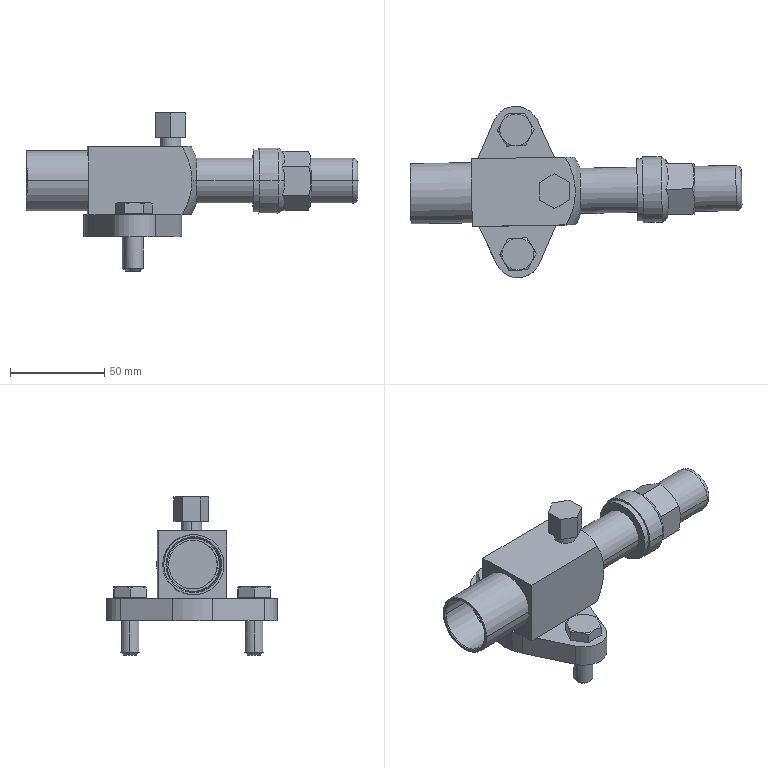Part | STEP file | 4PES-12Y-40P-1 | 1 solid | 138 faces | box 176.41 x 90.99 x 84 mm | volume 162399 mm3 | plane 60 | cylinder 39 | cone 19 | torus 18 | spline 2 | commonest cylinder face diameters 11 x6 10 x4 11.5 x4 24 x4 52 x3 25 x2